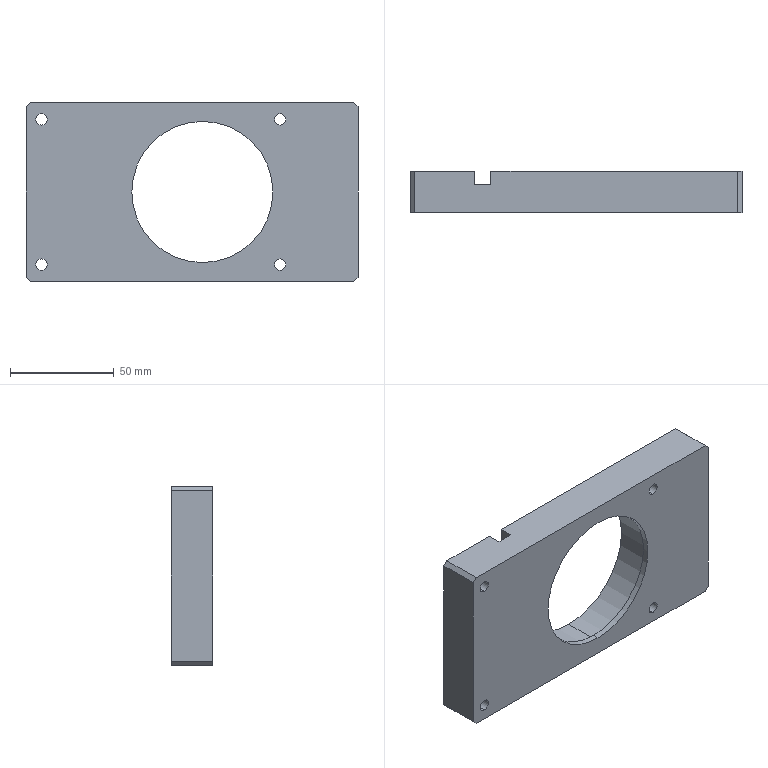Part | SolidWorks | features BaseBody 1 | 1 solid | 87 faces | box 160 x 20 x 86 mm | volume 181258 mm3 | cylinder 44 | plane 27 | cone 16 | commonest cylinder face diameters 2.5 x8 4 x8 5 x8 5.5 x8 10 x8 68 x2